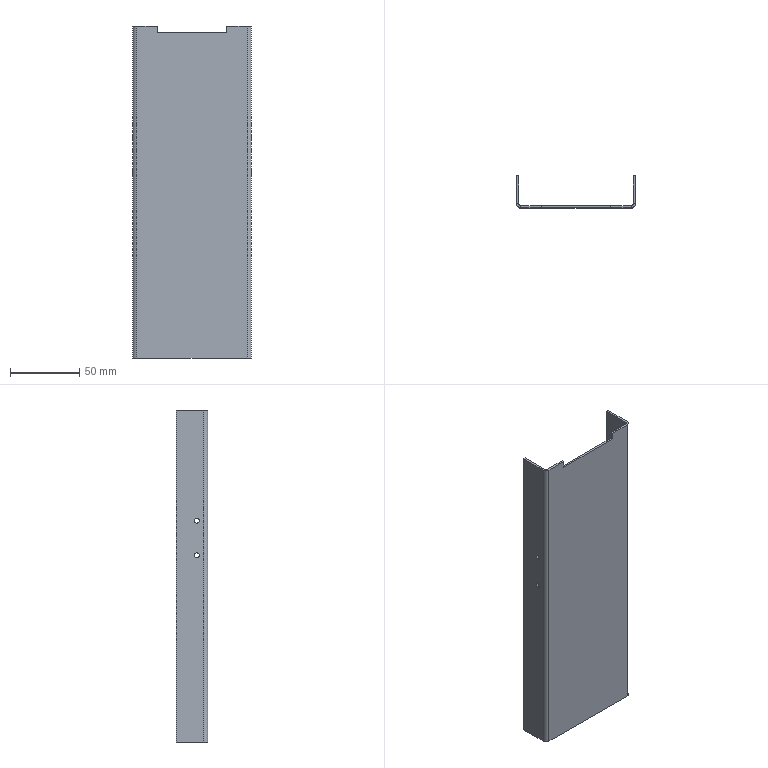Part | STEP file | Upper stop plate V1.201001 | 1 solid | 34 faces | box 86 x 23 x 240 mm | volume 45312 mm3 | plane 22 | cylinder 12 | commonest cylinder face diameters 3.5 x8 3 x2 6 x2